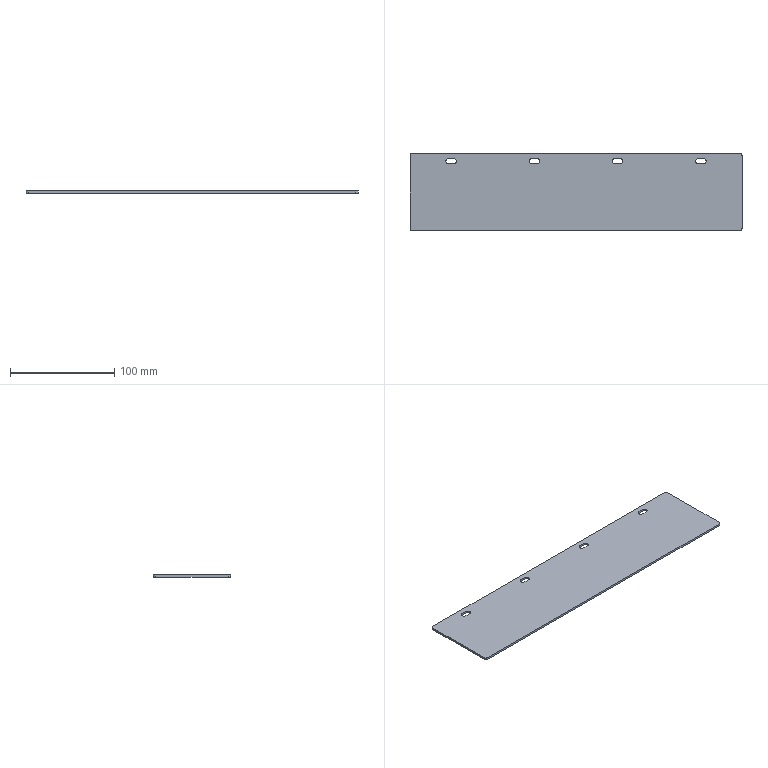Part | STEP file | 1 solid | 30 faces | box 319 x 74 x 2 mm | volume 46848 mm3 | cylinder 16 | plane 14 | commonest cylinder face diameters 5 x12 4 x4